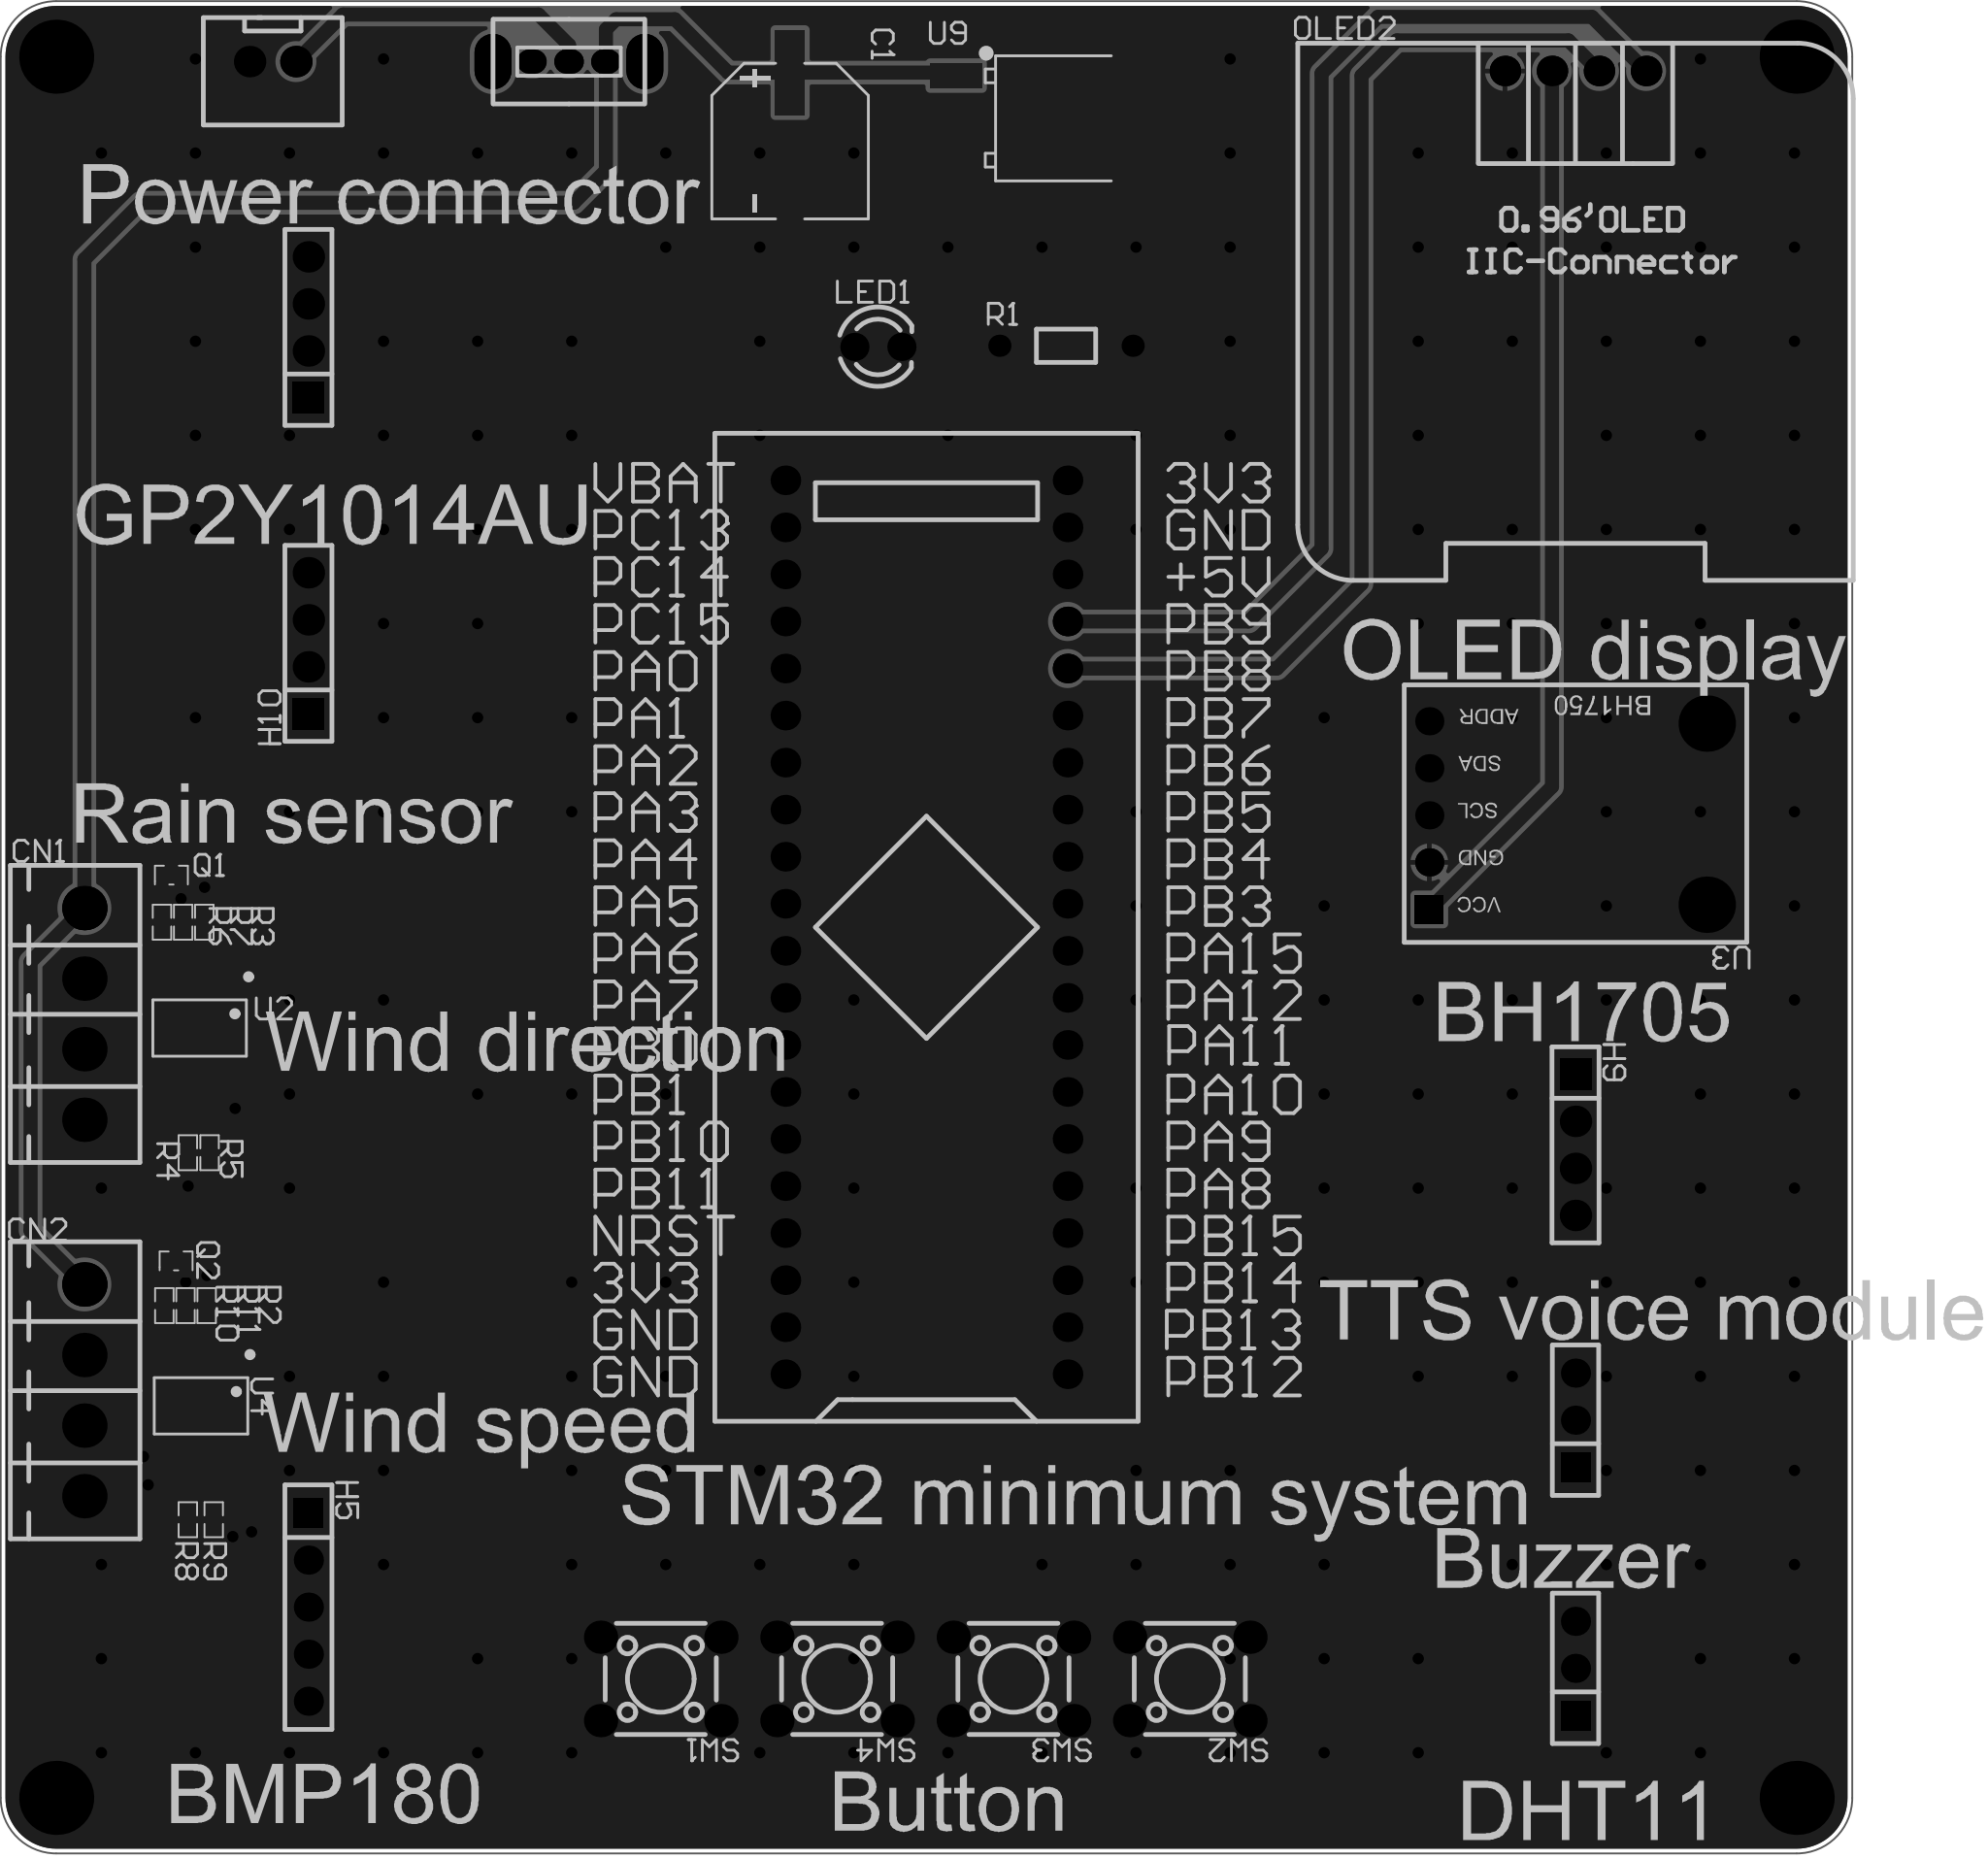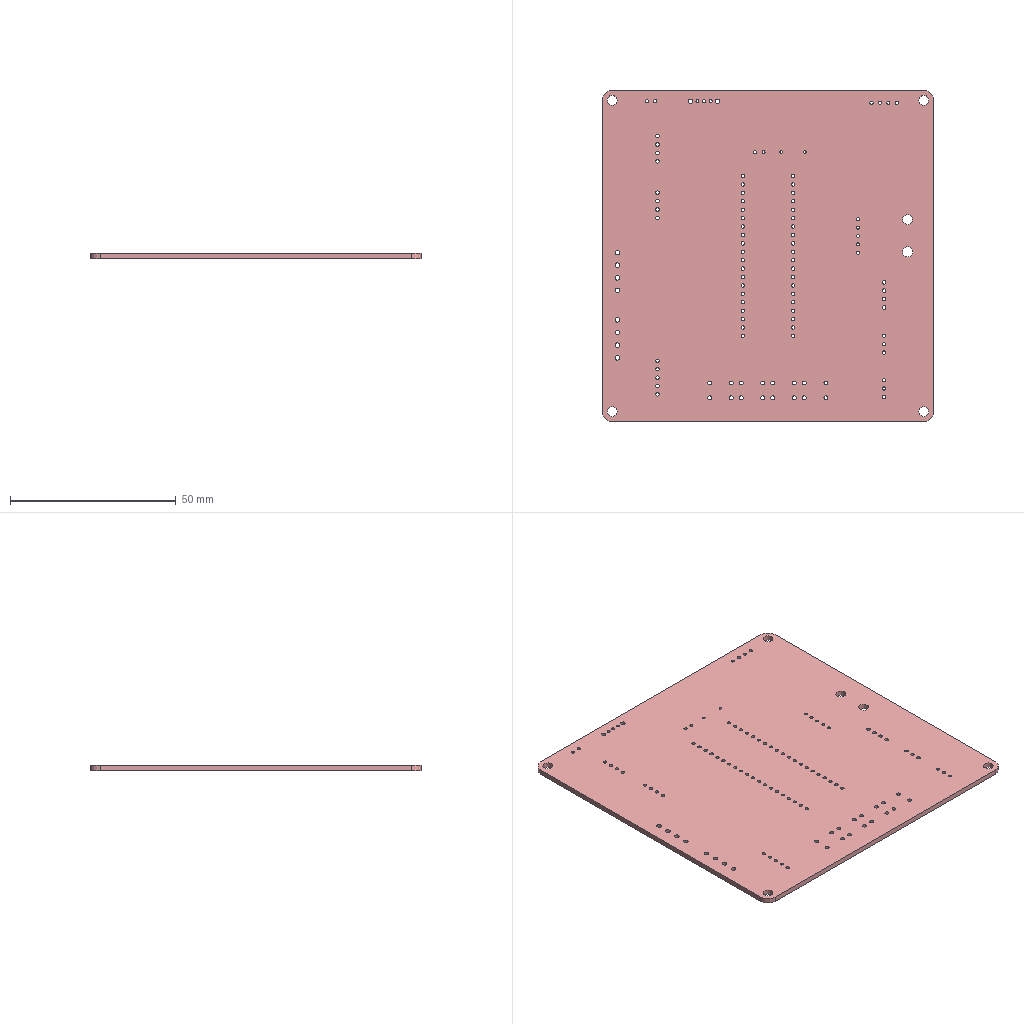Circuit board layout | Altium Designer | box 100 x 100 x 1.6 mm
Layer stack:
# Altium Designer layer stack of  (unit mm; dielectric type: 0 none, 1 core, 2 prepreg, 3 surface material)
index,name,kind,layer,copper_thickness_mm,dielectric_type,dielectric_thickness_mm,dielectric_material,dielectric_constant
0,Top Paste Mask Layer,other,,,,,,
1,Top Silkscreen Layer,other,,,,,,
2,Top Solder Mask Layer,dielectric,,,3,0.01,,3.3
3,Top Layer,copper,Top Layer,0.035,,,,
4,Dielectric1,dielectric,,,3,1.51,FR4,4.5
5,Bottom Layer,copper,Bottom Layer,0.035,,,,
6,Bottom Solder Mask Layer,dielectric,,,3,0.01,,3.3
7,Bottom Silkscreen Layer,other,,,,,,
8,Bottom Paste Mask Layer,other,,,,,,
# drill layer pairs: low layer,high layer
drill_pair,Top Layer,Bottom Layer
Part placement:
Designator,Comment,Layer,Footprint,Center-X(mm),Center-Y(mm),Rotation
U1,STM32F103C8T6-Card,TopLayer,CONN-TH_L53.3-W22.9_STM32F103C8T6-CARD,141.351,130.937,90
SW1,,TopLayer,SW-TH_4P-L6.0-W6.0-P4.50-LS6.5,127,90.36,180
SW2,,TopLayer,SW-TH_4P-L6.0-W6.0-P4.50-LS6.5,155.572,90.36,180
SW3,,TopLayer,SW-TH_4P-L6.0-W6.0-P4.50-LS6.5,146.048,90.36,180
SW4,,TopLayer,SW-TH_4P-L6.0-W6.0-P4.50-LS6.5,136.524,90.36,180
CN4,XH2.54*2P_through-hole,TopLayer,CONN-TH_2P-P2.50-XH2.54-2P,106.045,177.673,0
SW5,,TopLayer,拨动开关,122.039,177.673,180
H1,,TopLayer,HDR-TH_3P-P2.54-V-F,176.403,104.327,90
H3,,TopLayer,HDR-TH_3P-P2.54-V-F,176.403,90.929,90
H4,,TopLayer,HDR-TH_4P-P2.54-V-F,107.97,163.322,90
H5,,TopLayer,HDR-TH_5P-P2.54-V-F,107.97,94.234,270
OLED2,,TopLayer,0.96OLED_4P,176.403,177.165,0
C1,,TopLayer,CAP-SMD_BD8.0-L8.3-W8.3-LS9.3-FD,133.985,173.355,270
CN1,KF2EDGV-3.81-4P,TopLayer,CONN-TH_4P-P3.81_KF2EDGV-3.81-4P,95.871,126.26,270
CN2,KF2EDGV-3.81-4P,TopLayer,CONN-TH_4P-P3.81_KF2EDGV-3.81-4P,95.871,105.94,270
H9,,TopLayer,HDR-TH_4P-P2.54-V-F,176.403,119.191,270
H10,,TopLayer,HDR-TH_4P-P2.54-V-F,107.97,146.266,90
LED1,,TopLayer,LED_TH-3mm,138.729,162.268,0
Q1,S8050,TopLayer,SOT-523-3_L1.6-W0.8-P0.50-LS1.6-BR,100.57,133.753,270
Q2,S8050,TopLayer,SOT-523-3_L1.6-W0.8-P0.50-LS1.6-BR,100.824,112.925,270
R1,100,TopLayer,Res_1/8W,148.889,162.331,0
R2,4.7kΩ,TopLayer,R0402ST,102.475,110.512,270
R3,4.7kΩ,TopLayer,R0402ST,102.348,131.213,270
R4,4.7kΩ,TopLayer,R0402ST,101.459,118.767,270
R5,4.7kΩ,TopLayer,R0402ST,102.632,118.768,90
R6,1kΩ,TopLayer,R0402ST,100.062,131.213,270
R7,4.7kΩ,TopLayer,R0402ST,101.205,131.213,270
R8,4.7kΩ,TopLayer,R0402ST,101.459,98.955,270
R9,4.7kΩ,TopLayer,R0402ST,102.856,98.955,90
R10,1kΩ,TopLayer,R0402ST,100.189,110.512,270
R11,4.7kΩ,TopLayer,R0402ST,101.332,110.512,270
U2,XL3485,TopLayer,SOP-8_L5.0-W4.0-P1.27-LS6.0-BL,102.094,125.498,180
U3,,TopLayer,BH1750光照传感器,176.001,136.981,180
U4,XL3485,TopLayer,SOP-8_L5.0-W4.0-P1.27-LS6.0-BL,102.17,105.101,180
U9,L78M05ABDT-TR,TopLayer,TO-252-2_L6.5-W6.1-P4.58-LS10.0-TL,146.431,174.625,0
Pad and via stacks:
# Altium Designer via and pad stacks of  (unit mm). Each distinct definition once, with the count of objects using it.
# via: kind,start_layer,end_layer,hole_mm,diameter_mm,mode(0 simple;1 top-mid-bottom;2 full stack),diameter_per_layer,count,example_net
# pad: kind,layer,hole_mm,hole_type(0 round;1 square;2 slot),plating,top_size,top_shape(1 round;2 rect;3 octagon;9 rounded rect),mid_size,bottom_size,mode,footprint,size_per_layer,count,example
pad,Multi-Layer,3,0,plated,4x4,1,4x4,4x4,0,,,4,1
pad,Multi-Layer,1,0,plated,1.6x1.6,1,1.6x1.6,1.6x1.6,0,CONN-TH_L53.3-W22.9_STM32F103C8T6-CARD,,40,U1.1
pad,Multi-Layer,1.2,0,plated,1.8x1.8,1,1.8x1.8,1.8x1.8,0,SW-TH_4P-L6.0-W6.0-P4.50-LS6.5,,16,SW1.1
pad,Multi-Layer,1.05,0,plated,1.7x1.7,1,1.7x1.7,1.7x1.7,0,CONN-TH_2P-P2.50-XH2.54-2P,,2,CN4.2
pad,Multi-Layer,0.8992,0,plated,1.6x1.3,1,1.6x1.3,1.6x1.3,0,\u00B2\u00A6\u00B6\u00AF\u00BF\u00AA\u00B9\u00D8,,3,SW5.1
pad,Multi-Layer,1.3,0,plated,3x1.999,1,3x1.999,3x1.999,0,\u00B2\u00A6\u00B6\u00AF\u00BF\u00AA\u00B9\u00D8,,2,SW5.4
pad,Multi-Layer,1.02,0,plated,1.575x1.575,1,1.575x1.575,1.575x1.575,0,HDR-TH_3P-P2.54-V-F,,4,H1.3
pad,Multi-Layer,1.02,0,plated,1.575x1.575,2,1.575x1.575,1.575x1.575,0,HDR-TH_3P-P2.54-V-F,,2,H1.1
pad,Multi-Layer,1.1,0,plated,1.7x1.7,2,1.7x1.7,1.7x1.7,0,HDR-TH_4P-P2.54-V-F,,3,H4.1
pad,Multi-Layer,1.1,0,plated,1.7x1.7,1,1.7x1.7,1.7x1.7,0,HDR-TH_4P-P2.54-V-F,,9,H4.2
pad,Multi-Layer,1.02,0,plated,1.575x1.575,1,1.575x1.575,1.575x1.575,0,HDR-TH_5P-P2.54-V-F,,4,H5.5
pad,Multi-Layer,1.02,0,plated,1.575x1.575,2,1.575x1.575,1.575x1.575,0,HDR-TH_5P-P2.54-V-F,,1,H5.1
pad,Multi-Layer,1,0,plated,1.65x1.65,1,1.65x1.65,1.65x1.65,0,0.96OLED_4P,,4,OLED2.4
pad,Multi-Layer,1.4,0,plated,2.4x2.4,1,2.4x2.4,2.4x2.4,0,CONN-TH_4P-P3.81_KF2EDGV-3.81-4P,,8,CN1.2
pad,Multi-Layer,0.9144,0,plated,1.524x1.524,1,1.524x1.524,1.524x1.524,0,LED_TH-3mm,,2,LED1.1
pad,Multi-Layer,0.8001,0,plated,1.199x1.199,1,1.199x1.199,1.199x1.199,0,Res_1/8W,,2,R1.1
pad,Multi-Layer,3.048,0,unplated,3.048x3.048,1,3.048x3.048,3.048x3.048,0,BH1750\u00B9\u00E2\u00D5\u00D5\u00B4\u00AB\u00B8\u00D0\u00C6\u00F7,,2,U3.
pad,Multi-Layer,0.9144,0,plated,1.524x1.524,2,1.524x1.524,1.524x1.524,0,BH1750\u00B9\u00E2\u00D5\u00D5\u00B4\u00AB\u00B8\u00D0\u00C6\u00F7,,1,U3.1
pad,Multi-Layer,0.9144,0,plated,1.524x1.524,1,1.524x1.524,1.524x1.524,0,BH1750\u00B9\u00E2\u00D5\u00D5\u00B4\u00AB\u00B8\u00D0\u00C6\u00F7,,4,U3.4
pad,Top Layer,0,0,plated,4.6x1.6,2,4.6x1.6,4.6x1.6,0,CAP-SMD_BD8.0-L8.3-W8.3-LS9.3-FD,,2,C1.1
pad,Top Layer,0,0,plated,0.51x0.4,2,0.51x0.4,0.51x0.4,0,SOT-523-3_L1.6-W0.8-P0.50-LS1.6-BR,,6,Q1.1
pad,Top Layer,0,0,plated,0.5657x0.54,2,0.5657x0.54,0.5657x0.54,0,R0402ST,,20,R2.2
pad,Top Layer,0,0,plated,0.574x2.035,1,0.574x2.035,0.574x2.035,0,SOP-8_L5.0-W4.0-P1.27-LS6.0-BL,,16,U2.1
pad,Top Layer,0,0,plated,6.5x6,2,6.5x6,6.5x6,0,TO-252-2_L6.5-W6.1-P4.58-LS10.0-TL,,1,U9.4
pad,Top Layer,0,0,plated,2.8x1.35,2,2.8x1.35,2.8x1.35,0,TO-252-2_L6.5-W6.1-P4.58-LS10.0-TL,,1,U9.1
pad,Top Layer,0,0,plated,2.8x1.5,2,2.8x1.5,2.8x1.5,0,TO-252-2_L6.5-W6.1-P4.58-LS10.0-TL,,1,U9.3
via,Top Layer,Bottom Layer,0.3048,0.61,0,,207,VCC
Copper pours:
name,layer,net,type(0 solid;1 hatched;2 none)
Bottom Layer-GND,Bottom Layer,GND,0
Top Layer-GND,Top Layer,GND,0
Design rules, without the lines most boards share:
# Altium Designer design rules of  (exported by Altium Designer, unit mm)
# columns: name | kind | enabled | priority | scope1 | scope2 | descriptor | typed fields (field=value)
Copper_copperRegion_copperThickness1oz | 0 | disabled | 4 | All | All | Clearance Constraint (Gap=5.984mil) (Disabled)(All),(All) | gap=0.152
Copper_copperRegion_copperThickness1oz_1 | 63 | disabled | 4 | All | All | Board Clearance Constraint (Gap=0mil) (Disabled)(All) |
Copper_copperRegion_Copper_copperRegion | 0 | disabled | 5 | All | All | Clearance Constraint (Gap=5.984mil) (Disabled)(All),(All) | gap=0.152
Copper_copperRegion_Copper_copperRegion_1 | 63 | disabled | 5 | All | All | Board Clearance Constraint (Gap=0mil) (Disabled)(All) |
copperThickness1oz | 0 | enabled | 6 | All | All | Clearance Constraint (Gap=5.984mil) (All),(All) | gap=0.152
copperThickness1oz_1 | 63 | enabled | 6 | All | All | Board Clearance Constraint (Gap=0mil) (All) |
copperRegion_copperThickness1oz | 20 | disabled | 1 | All | All | Polygon Connect Rule(Relief Connect )(Conductor Width=10mil) (Relief Angle=90 Angle) (Entries=4) (Air Gap Width=10mil) (Disabled)(All),(All) | connect_style(0=relief,1=direct,2=none)=0 relief_conductor_width=0.254 relief_entries=4
copperRegion_Copper_copperRegion | 20 | disabled | 2 | All | All | Polygon Connect Rule(Relief Connect )(Conductor Width=10mil) (Relief Angle=90 Angle) (Entries=4) (Air Gap Width=10mil) (Disabled)(All),(All) | connect_style(0=relief,1=direct,2=none)=0 relief_conductor_width=0.254 relief_entries=4
copperRegion | 20 | enabled | 3 | All | All | Polygon Connect Rule(Relief Connect )(Conductor Width=10mil) (Relief Angle=90 Angle) (Entries=4) (Air Gap Width=10mil) (All),(All) | connect_style(0=relief,1=direct,2=none)=0 relief_conductor_width=0.254 relief_entries=4